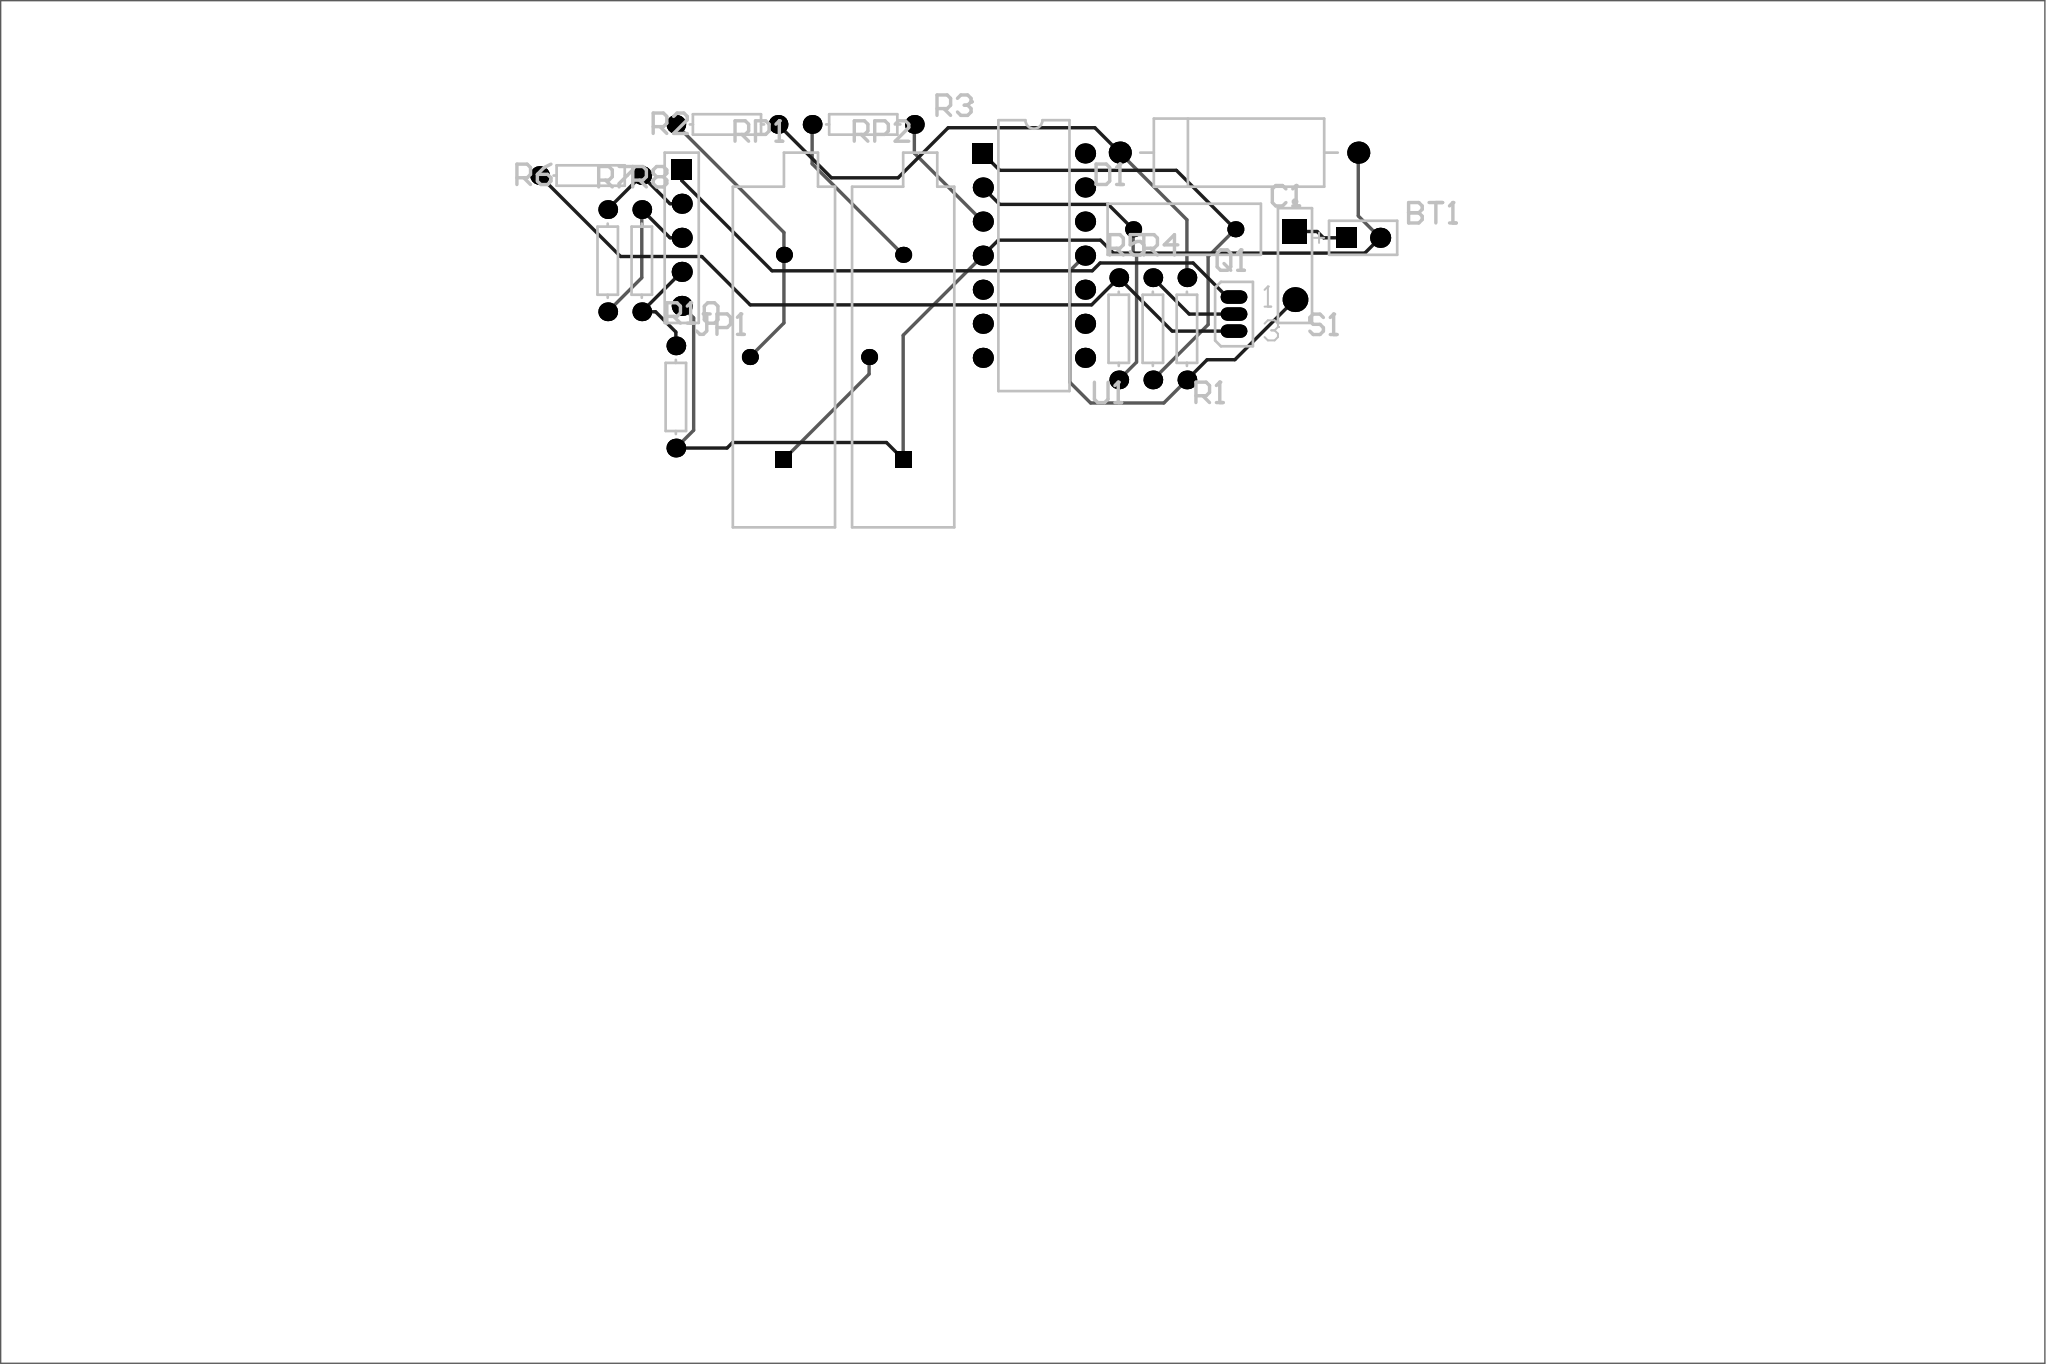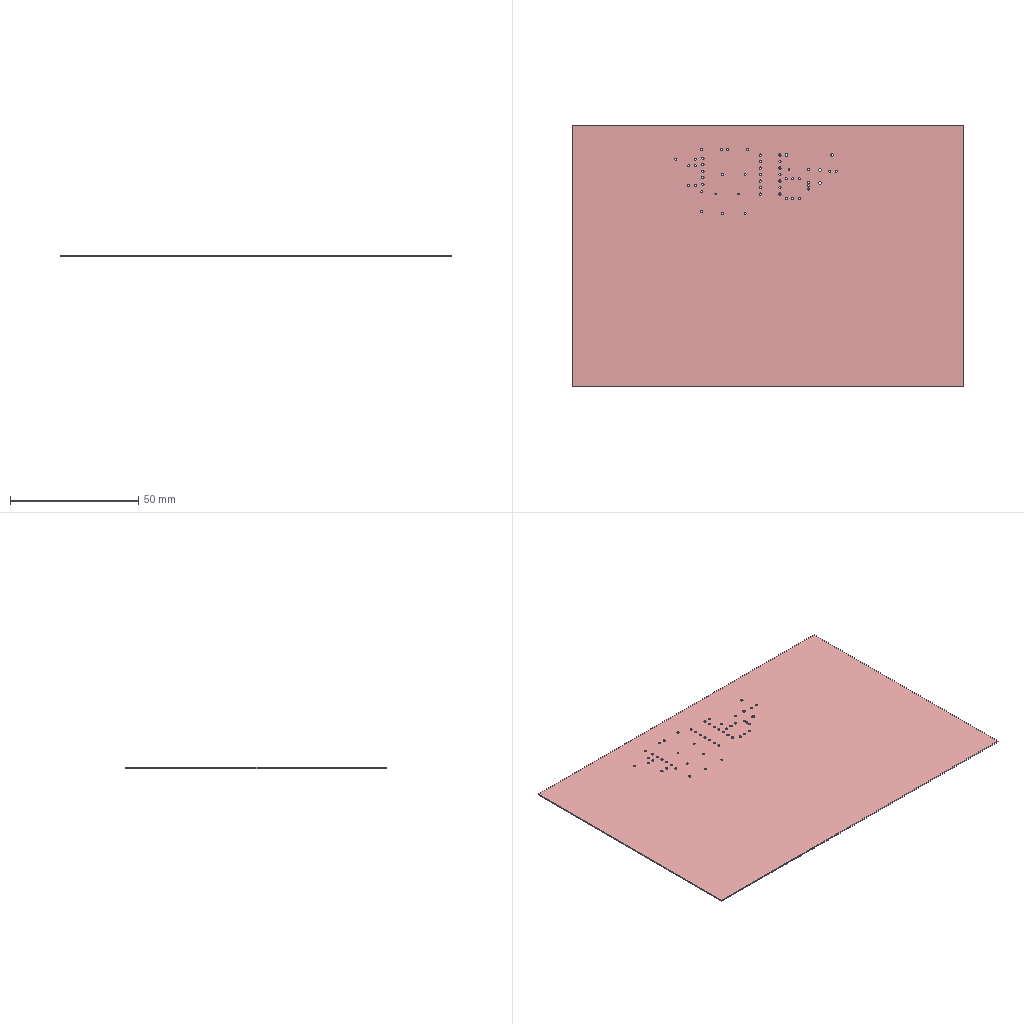Circuit board layout | Altium Designer | box 152.4 x 101.6 x 0.4 mm
Layer stack:
# Altium Designer layer stack of  (unit mm; dielectric type: 0 none, 1 core, 2 prepreg, 3 surface material)
index,name,kind,layer,copper_thickness_mm,dielectric_type,dielectric_thickness_mm,dielectric_material,dielectric_constant
0,Top Paste,other,,,,,,
1,Top Overlay,other,,,,,,
2,Top Solder,dielectric,,,3,0.0102,Solder Resist,3.5
3,Top Layer,copper,Top Layer,0.0356,,,,
4,Dielectric1,dielectric,,,0,0.32,FR-4,4.8
5,Bottom Layer,copper,Bottom Layer,0.0356,,,,
6,Bottom Solder,dielectric,,,3,0.0102,Solder Resist,3.5
7,Bottom Overlay,other,,,,,,
8,Bottom Paste,other,,,,,,
# drill layer pairs: low layer,high layer
drill_pair,Top Layer,Bottom Layer
Part placement:
Designator,Comment,Layer,Footprint,Center-X(mm),Center-Y(mm),Rotation
BT1,Battery,TopLayer,BAT-2,126.973,109.32,360
C1,Cap,TopLayer,RAD-0.3,113.638,109.955,360
D1,D Zener,TopLayer,DIODE-0.7,117.721,115.67,180
JP1,Header 5,TopLayer,HDR1X5,76.173,109.32,270
Q1,MOSFET-N,TopLayer,BCY-W3/H.8,117.348,103.632,360
R1,Res1,TopLayer,AXIAL-0.3,113.836,102.533,270
R2,Res1,TopLayer,AXIAL-0.3,79.546,117.773,180
R3,Res1,TopLayer,AXIAL-0.3,89.706,117.773,360
R4,Res1,TopLayer,AXIAL-0.3,111.296,102.533,90
R5,Res1,TopLayer,AXIAL-0.3,108.756,102.533,90
R6,Res1,TopLayer,AXIAL-0.3,69.386,113.963,180
R7,Res1,TopLayer,AXIAL-0.3,70.656,107.613,90
R8,Res1,TopLayer,AXIAL-0.3,73.196,107.613,90
R10,Res1,TopLayer,AXIAL-0.3,75.736,97.453,90
RP1,RPot,TopLayer,VR2,82.523,100.43,90
RP2,RPot,TopLayer,VR2,91.413,100.43,90
S1,SW-SPST,TopLayer,SPST-2,121.893,107.25,270
U1,LM248J,TopLayer,J014,102.431,107.99,270
Pad and via stacks:
# Altium Designer via and pad stacks of  (unit mm). Each distinct definition once, with the count of objects using it.
# via: kind,start_layer,end_layer,hole_mm,diameter_mm,mode(0 simple;1 top-mid-bottom;2 full stack),diameter_per_layer,count,example_net
# pad: kind,layer,hole_mm,hole_type(0 round;1 square;2 slot),plating,top_size,top_shape(1 round;2 rect;3 octagon;9 rounded rect),mid_size,bottom_size,mode,footprint,size_per_layer,count,example
pad,Multi-Layer,0.7,0,plated,1.2x1.2,2,1.2x1.2,1.2x1.2,0,VR2,,2,RP1.1
pad,Multi-Layer,0.7,0,plated,1.2x1.2,1,1.2x1.2,1.2x1.2,0,VR2,,4,RP1.3
pad,Multi-Layer,0.9,0,plated,1.5x1.5,2,1.5x1.5,1.5x1.5,0,J014,,1,U1.1
pad,Multi-Layer,0.9,0,plated,1.5x1.5,1,1.5x1.5,1.5x1.5,0,J014,,13,U1.2
pad,Multi-Layer,1,0,plated,1.65x1.65,1,1.65x1.65,1.65x1.65,0,DIODE-0.7,,2,D1.2
pad,Multi-Layer,0.7,0,plated,1.2x1.2,1,1.2x1.2,1.2x1.2,0,RAD-0.3,,2,C1.1
pad,Multi-Layer,0.9,0,plated,1.5x1.5,1,1.5x1.5,1.5x1.5,0,HDR1X5,,4,JP1.5
pad,Multi-Layer,0.9,0,plated,1.5x1.5,2,1.5x1.5,1.5x1.5,0,HDR1X5,,1,JP1.1
pad,Multi-Layer,1.1,0,plated,1.85x1.85,2,1.85x1.85,1.85x1.85,0,SPST-2,,1,S1.1
pad,Multi-Layer,1.1,0,plated,1.85x1.85,1,1.85x1.85,1.85x1.85,0,SPST-2,,1,S1.2
pad,Multi-Layer,0.85,0,plated,1.4x1.4,1,1.4x1.4,1.4x1.4,0,AXIAL-0.3,,18,R3.2
pad,Multi-Layer,0.8,0,plated,2x1,1,2x1,2x1,0,BCY-W3/H.8,,3,Q1.1
pad,Multi-Layer,0.9,0,plated,1.5x1.5,2,1.5x1.5,1.5x1.5,0,BAT-2,,1,BT1.1
pad,Multi-Layer,0.9,0,plated,1.5x1.5,1,1.5x1.5,1.5x1.5,0,BAT-2,,1,BT1.2
Design rules, without the lines most boards share:
# Altium Designer design rules of  (exported by Altium Designer, unit mm)
# columns: name | kind | enabled | priority | scope1 | scope2 | descriptor | typed fields (field=value)
HoleToHoleClearance | 52 | enabled | 1 | All | All | Hole To Hole Clearance (Gap=10mil) (All),(All) | gap=0.254
DiffPairsRouting | 51 | enabled | 1 | All | All | Differential Pairs Uncoupled Length using the Gap Constraints (Min=10mil) (Max=10mil) (Prefered=10mil)  and Width Constraints (Min=15mil) (Max=15mil) (Prefered=15mil) (All) |
Testpoint | 43 | enabled | 1 | All | All | Fabrication Testpoint Style (Under Component=Yes) (All) |
TestPointUsage | 44 | enabled | 1 | All | All | Fabrication Testpoint Usage (Valid =One Required, Allow multiple per net=No) (All) |
SolderMaskExpansion | 13 | enabled | 1 | All | All | Solder Mask Expansion (Expansion =4mil) (All) | expansion=0.1016
PasteMaskExpansion | 14 | enabled | 1 | All | All | Paste Mask Expansion (Expansion =0mil) (All) | expansion=0
RoutingVias | 11 | enabled | 1 | All | All | Routing Via (MinHoleWidth=28mil) (MaxHoleWidth=28mil) (PreferredHoleWidth=28mil) (MinWidth=50mil) (MaxWidth=50mil) (PreferedWidth=50mil) (All) | via_min_hole=0.7112 via_max_hole=0.7112 via_preferred_diameter=1.27 via_preferred_hole=0.7112
Width | 2 | enabled | 1 | All | All | Width Constraint (Min=10mil) (Max=10mil) (Preferred=10mil) (All) |
PolygonConnect | 20 | enabled | 1 | All | All | Polygon Connect Rule(Relief Connect )(Conductor Width=10mil) (Relief Angle=90 Angle) (Entries=4) (Air Gap Width=10mil) (All),(All) | connect_style(0=relief,1=direct,2=none)=0 relief_conductor_width=0.254 relief_entries=4
PlaneConnect | 6 | enabled | 1 | All | All | Power Plane Connect Rule(Relief Connect )(Expansion=20mil) (Conductor Width=10mil) (Air Gap=10mil) (Entries=4) (All) | relief_conductor_width=0.254 relief_entries=4 relief_expansion=0.508
Clearance | 0 | enabled | 1 | All | All | Clearance Constraint (Gap=10mil) (All),(All) | gap=0.254